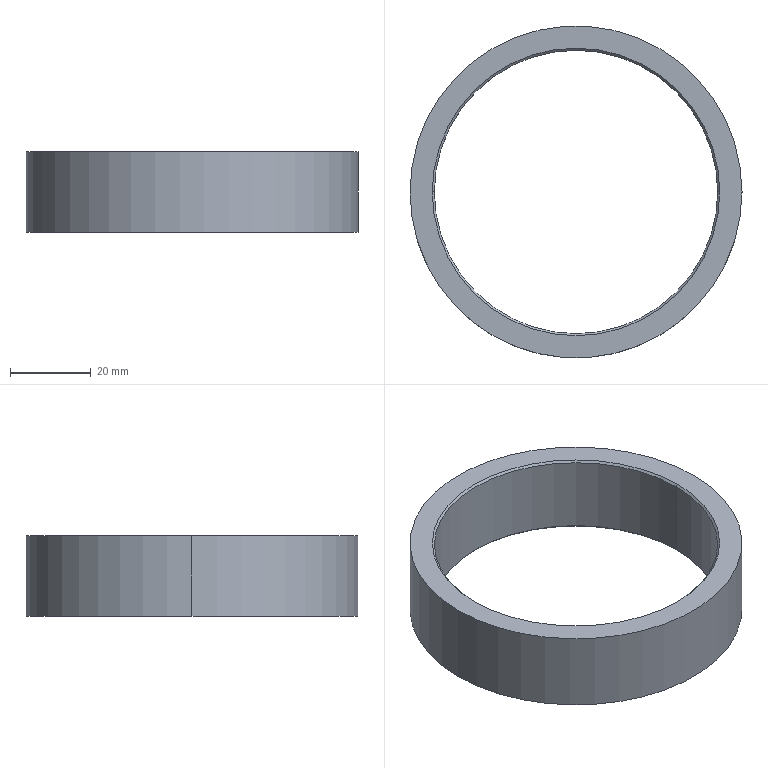Part | SolidWorks | features Chamfer 1, Extrusion 1 | 1 solid | 10 faces | box 82 x 82 x 20 mm | volume 28596 mm3 | cone 4 | cylinder 4 | plane 2 | commonest cylinder face diameters 70 x2 82 x2
STEP:
#1=CARTESIAN_POINT('',(35.,0.,0.5));
#2=VERTEX_POINT('',#1);
#3=CARTESIAN_POINT('',(-35.,0.,0.5));
#4=VERTEX_POINT('',#3);
#5=CARTESIAN_POINT('',(0.,0.,0.5));
#6=DIRECTION('',(0.,0.,-1.));
#7=DIRECTION('',(1.,0.,0.));
#8=AXIS2_PLACEMENT_3D('',#5,#6,#7);
#9=CIRCLE('',#8,35.);
#10=EDGE_CURVE('',#2,#4,#9,.T.);
#11=ORIENTED_EDGE('',*,*,#10,.F.);
#12=CARTESIAN_POINT('',(35.5,0.,0.));
#13=VERTEX_POINT('',#12);
#14=CARTESIAN_POINT('',(35.5,0.,0.));
#15=DIRECTION('',(0.7071,0.,-0.7071));
#16=VECTOR('',#15,1000.);
#17=LINE('',#14,#16);
#18=EDGE_CURVE('',#2,#13,#17,.T.);
#19=ORIENTED_EDGE('',*,*,#18,.T.);
#20=CARTESIAN_POINT('',(-35.5,0.,0.));
#21=VERTEX_POINT('',#20);
#22=CARTESIAN_POINT('',(0.,0.,0.));
#23=DIRECTION('',(0.,0.,1.));
#24=DIRECTION('',(1.,0.,0.));
#25=AXIS2_PLACEMENT_3D('',#22,#23,#24);
#26=CIRCLE('',#25,35.5);
#27=EDGE_CURVE('',#21,#13,#26,.T.);
#28=ORIENTED_EDGE('',*,*,#27,.F.);
#29=CARTESIAN_POINT('',(-35.5,0.,0.));
#30=DIRECTION('',(-0.7071,0.,-0.7071));
#31=VECTOR('',#30,1000.);
#32=LINE('',#29,#31);
#33=EDGE_CURVE('',#4,#21,#32,.T.);
#34=ORIENTED_EDGE('',*,*,#33,.F.);
#35=EDGE_LOOP('',(#11,#19,#28,#34));
#36=FACE_OUTER_BOUND('',#35,.T.);
#37=CARTESIAN_POINT('',(0.,0.,0.));
#38=DIRECTION('',(0.,0.,-1.));
#39=DIRECTION('',(-1.,0.,0.));
#40=AXIS2_PLACEMENT_3D('',#37,#38,#39);
#41=CONICAL_SURFACE('',#40,35.5,0.7854);
#42=ADVANCED_FACE('',(#36),#41,.F.);
#43=CARTESIAN_POINT('',(-35.,0.,19.5));
#44=VERTEX_POINT('',#43);
#45=CARTESIAN_POINT('',(35.,0.,19.5));
#46=VERTEX_POINT('',#45);
#47=CARTESIAN_POINT('',(0.,0.,19.5));
#48=DIRECTION('',(0.,0.,1.));
#49=DIRECTION('',(1.,0.,0.));
#50=AXIS2_PLACEMENT_3D('',#47,#48,#49);
#51=CIRCLE('',#50,35.);
#52=EDGE_CURVE('',#44,#46,#51,.T.);
#53=ORIENTED_EDGE('',*,*,#52,.F.);
#54=CARTESIAN_POINT('',(-35.5,0.,20.));
#55=VERTEX_POINT('',#54);
#56=CARTESIAN_POINT('',(-35.,0.,19.5));
#57=DIRECTION('',(-0.7071,0.,0.7071));
#58=VECTOR('',#57,1000.);
#59=LINE('',#56,#58);
#60=EDGE_CURVE('',#44,#55,#59,.T.);
#61=ORIENTED_EDGE('',*,*,#60,.T.);
#62=CARTESIAN_POINT('',(35.5,0.,20.));
#63=VERTEX_POINT('',#62);
#64=CARTESIAN_POINT('',(0.,0.,20.));
#65=DIRECTION('',(0.,0.,-1.));
#66=DIRECTION('',(1.,0.,0.));
#67=AXIS2_PLACEMENT_3D('',#64,#65,#66);
#68=CIRCLE('',#67,35.5);
#69=EDGE_CURVE('',#63,#55,#68,.T.);
#70=ORIENTED_EDGE('',*,*,#69,.F.);
#71=CARTESIAN_POINT('',(35.,0.,19.5));
#72=DIRECTION('',(0.7071,0.,0.7071));
#73=VECTOR('',#72,1000.);
#74=LINE('',#71,#73);
#75=EDGE_CURVE('',#46,#63,#74,.T.);
#76=ORIENTED_EDGE('',*,*,#75,.F.);
#77=EDGE_LOOP('',(#53,#61,#70,#76));
#78=FACE_OUTER_BOUND('',#77,.T.);
#79=CARTESIAN_POINT('',(0.,0.,19.5));
#80=DIRECTION('',(0.,0.,1.));
#81=DIRECTION('',(1.,0.,0.));
#82=AXIS2_PLACEMENT_3D('',#79,#80,#81);
#83=CONICAL_SURFACE('',#82,35.,0.7854);
#84=ADVANCED_FACE('',(#78),#83,.F.);
#85=ORIENTED_EDGE('',*,*,#52,.T.);
#86=CARTESIAN_POINT('',(35.,0.,20.));
#87=DIRECTION('',(0.,0.,-1.));
#88=VECTOR('',#87,1000.);
#89=LINE('',#86,#88);
#90=EDGE_CURVE('',#46,#2,#89,.T.);
#91=ORIENTED_EDGE('',*,*,#90,.T.);
#92=ORIENTED_EDGE('',*,*,#10,.T.);
#93=CARTESIAN_POINT('',(-35.,0.,20.));
#94=DIRECTION('',(0.,0.,-1.));
#95=VECTOR('',#94,1000.);
#96=LINE('',#93,#95);
#97=EDGE_CURVE('',#44,#4,#96,.T.);
#98=ORIENTED_EDGE('',*,*,#97,.F.);
#99=EDGE_LOOP('',(#85,#91,#92,#98));
#100=FACE_OUTER_BOUND('',#99,.T.);
#101=CARTESIAN_POINT('',(0.,0.,20.));
#102=DIRECTION('',(0.,0.,-1.));
#103=DIRECTION('',(-1.,0.,0.));
#104=AXIS2_PLACEMENT_3D('',#101,#102,#103);
#105=CYLINDRICAL_SURFACE('',#104,35.);
#106=ADVANCED_FACE('',(#100),#105,.F.);
#107=CARTESIAN_POINT('',(41.,0.,20.));
#108=VERTEX_POINT('',#107);
#109=CARTESIAN_POINT('',(-41.,0.,20.));
#110=VERTEX_POINT('',#109);
#111=CARTESIAN_POINT('',(0.,0.,20.));
#112=DIRECTION('',(0.,0.,1.));
#113=DIRECTION('',(1.,0.,0.));
#114=AXIS2_PLACEMENT_3D('',#111,#112,#113);
#115=CIRCLE('',#114,41.);
#116=EDGE_CURVE('',#108,#110,#115,.T.);
#117=ORIENTED_EDGE('',*,*,#116,.F.);
#118=CARTESIAN_POINT('',(41.,0.,0.));
#119=VERTEX_POINT('',#118);
#120=CARTESIAN_POINT('',(41.,0.,20.));
#121=DIRECTION('',(0.,0.,-1.));
#122=VECTOR('',#121,1000.);
#123=LINE('',#120,#122);
#124=EDGE_CURVE('',#108,#119,#123,.T.);
#125=ORIENTED_EDGE('',*,*,#124,.T.);
#126=CARTESIAN_POINT('',(-41.,0.,0.));
#127=VERTEX_POINT('',#126);
#128=CARTESIAN_POINT('',(0.,0.,0.));
#129=DIRECTION('',(0.,0.,1.));
#130=DIRECTION('',(1.,0.,0.));
#131=AXIS2_PLACEMENT_3D('',#128,#129,#130);
#132=CIRCLE('',#131,41.);
#133=EDGE_CURVE('',#119,#127,#132,.T.);
#134=ORIENTED_EDGE('',*,*,#133,.T.);
#135=CARTESIAN_POINT('',(-41.,0.,20.));
#136=DIRECTION('',(0.,0.,-1.));
#137=VECTOR('',#136,1000.);
#138=LINE('',#135,#137);
#139=EDGE_CURVE('',#110,#127,#138,.T.);
#140=ORIENTED_EDGE('',*,*,#139,.F.);
#141=EDGE_LOOP('',(#117,#125,#134,#140));
#142=FACE_OUTER_BOUND('',#141,.T.);
#143=CARTESIAN_POINT('',(0.,0.,20.));
#144=DIRECTION('',(0.,0.,-1.));
#145=DIRECTION('',(-1.,0.,0.));
#146=AXIS2_PLACEMENT_3D('',#143,#144,#145);
#147=CYLINDRICAL_SURFACE('',#146,41.);
#148=ADVANCED_FACE('',(#142),#147,.T.);
#149=ORIENTED_EDGE('',*,*,#69,.T.);
#150=CARTESIAN_POINT('',(0.,0.,20.));
#151=DIRECTION('',(0.,0.,-1.));
#152=DIRECTION('',(1.,0.,0.));
#153=AXIS2_PLACEMENT_3D('',#150,#151,#152);
#154=CIRCLE('',#153,35.5);
#155=EDGE_CURVE('',#55,#63,#154,.T.);
#156=ORIENTED_EDGE('',*,*,#155,.T.);
#157=EDGE_LOOP('',(#149,#156));
#158=FACE_BOUND('',#157,.T.);
#159=CARTESIAN_POINT('',(0.,0.,20.));
#160=DIRECTION('',(0.,0.,1.));
#161=DIRECTION('',(1.,0.,0.));
#162=AXIS2_PLACEMENT_3D('',#159,#160,#161);
#163=CIRCLE('',#162,41.);
#164=EDGE_CURVE('',#110,#108,#163,.T.);
#165=ORIENTED_EDGE('',*,*,#164,.T.);
#166=ORIENTED_EDGE('',*,*,#116,.T.);
#167=EDGE_LOOP('',(#165,#166));
#168=FACE_OUTER_BOUND('',#167,.T.);
#169=CARTESIAN_POINT('',(0.,0.,20.));
#170=DIRECTION('',(0.,0.,1.));
#171=DIRECTION('',(1.,0.,0.));
#172=AXIS2_PLACEMENT_3D('',#169,#170,#171);
#173=PLANE('',#172);
#174=ADVANCED_FACE('',(#158,#168),#173,.T.);
#175=ORIENTED_EDGE('',*,*,#27,.T.);
#176=CARTESIAN_POINT('',(0.,0.,0.));
#177=DIRECTION('',(0.,0.,1.));
#178=DIRECTION('',(1.,0.,0.));
#179=AXIS2_PLACEMENT_3D('',#176,#177,#178);
#180=CIRCLE('',#179,35.5);
#181=EDGE_CURVE('',#13,#21,#180,.T.);
#182=ORIENTED_EDGE('',*,*,#181,.T.);
#183=EDGE_LOOP('',(#175,#182));
#184=FACE_BOUND('',#183,.T.);
#185=CARTESIAN_POINT('',(0.,0.,0.));
#186=DIRECTION('',(0.,0.,1.));
#187=DIRECTION('',(1.,0.,0.));
#188=AXIS2_PLACEMENT_3D('',#185,#186,#187);
#189=CIRCLE('',#188,41.);
#190=EDGE_CURVE('',#127,#119,#189,.T.);
#191=ORIENTED_EDGE('',*,*,#190,.F.);
#192=ORIENTED_EDGE('',*,*,#133,.F.);
#193=EDGE_LOOP('',(#191,#192));
#194=FACE_OUTER_BOUND('',#193,.T.);
#195=CARTESIAN_POINT('',(0.,0.,0.));
#196=DIRECTION('',(0.,0.,1.));
#197=DIRECTION('',(1.,0.,0.));
#198=AXIS2_PLACEMENT_3D('',#195,#196,#197);
#199=PLANE('',#198);
#200=ADVANCED_FACE('',(#184,#194),#199,.F.);
#201=ORIENTED_EDGE('',*,*,#124,.F.);
#202=ORIENTED_EDGE('',*,*,#164,.F.);
#203=ORIENTED_EDGE('',*,*,#139,.T.);
#204=ORIENTED_EDGE('',*,*,#190,.T.);
#205=EDGE_LOOP('',(#201,#202,#203,#204));
#206=FACE_OUTER_BOUND('',#205,.T.);
#207=CARTESIAN_POINT('',(0.,0.,20.));
#208=DIRECTION('',(0.,0.,-1.));
#209=DIRECTION('',(-1.,0.,0.));
#210=AXIS2_PLACEMENT_3D('',#207,#208,#209);
#211=CYLINDRICAL_SURFACE('',#210,41.);
#212=ADVANCED_FACE('',(#206),#211,.T.);
#213=ORIENTED_EDGE('',*,*,#90,.F.);
#214=CARTESIAN_POINT('',(0.,0.,19.5));
#215=DIRECTION('',(0.,0.,1.));
#216=DIRECTION('',(1.,0.,0.));
#217=AXIS2_PLACEMENT_3D('',#214,#215,#216);
#218=CIRCLE('',#217,35.);
#219=EDGE_CURVE('',#46,#44,#218,.T.);
#220=ORIENTED_EDGE('',*,*,#219,.T.);
#221=ORIENTED_EDGE('',*,*,#97,.T.);
#222=CARTESIAN_POINT('',(0.,0.,0.5));
#223=DIRECTION('',(0.,0.,-1.));
#224=DIRECTION('',(1.,0.,0.));
#225=AXIS2_PLACEMENT_3D('',#222,#223,#224);
#226=CIRCLE('',#225,35.);
#227=EDGE_CURVE('',#4,#2,#226,.T.);
#228=ORIENTED_EDGE('',*,*,#227,.T.);
#229=EDGE_LOOP('',(#213,#220,#221,#228));
#230=FACE_OUTER_BOUND('',#229,.T.);
#231=CARTESIAN_POINT('',(0.,0.,20.));
#232=DIRECTION('',(0.,0.,-1.));
#233=DIRECTION('',(-1.,0.,0.));
#234=AXIS2_PLACEMENT_3D('',#231,#232,#233);
#235=CYLINDRICAL_SURFACE('',#234,35.);
#236=ADVANCED_FACE('',(#230),#235,.F.);
#237=ORIENTED_EDGE('',*,*,#60,.F.);
#238=ORIENTED_EDGE('',*,*,#219,.F.);
#239=ORIENTED_EDGE('',*,*,#75,.T.);
#240=ORIENTED_EDGE('',*,*,#155,.F.);
#241=EDGE_LOOP('',(#237,#238,#239,#240));
#242=FACE_OUTER_BOUND('',#241,.T.);
#243=CARTESIAN_POINT('',(0.,0.,19.5));
#244=DIRECTION('',(0.,0.,1.));
#245=DIRECTION('',(1.,0.,0.));
#246=AXIS2_PLACEMENT_3D('',#243,#244,#245);
#247=CONICAL_SURFACE('',#246,35.,0.7854);
#248=ADVANCED_FACE('',(#242),#247,.F.);
#249=ORIENTED_EDGE('',*,*,#18,.F.);
#250=ORIENTED_EDGE('',*,*,#227,.F.);
#251=ORIENTED_EDGE('',*,*,#33,.T.);
#252=ORIENTED_EDGE('',*,*,#181,.F.);
#253=EDGE_LOOP('',(#249,#250,#251,#252));
#254=FACE_OUTER_BOUND('',#253,.T.);
#255=CARTESIAN_POINT('',(0.,0.,0.));
#256=DIRECTION('',(0.,0.,-1.));
#257=DIRECTION('',(-1.,0.,0.));
#258=AXIS2_PLACEMENT_3D('',#255,#256,#257);
#259=CONICAL_SURFACE('',#258,35.5,0.7854);
#260=ADVANCED_FACE('',(#254),#259,.F.);
#261=CLOSED_SHELL('',(#42,#84,#106,#148,#174,#200,#212,#236,#248,#260));
#262=MANIFOLD_SOLID_BREP('',#261);
#263=CARTESIAN_POINT('',(0.,0.,0.));
#264=DIRECTION('',(0.,0.,1.));
#265=DIRECTION('',(1.,0.,0.));
#266=AXIS2_PLACEMENT_3D('',#263,#264,#265);
#267=(LENGTH_UNIT()NAMED_UNIT(*)SI_UNIT(.MILLI.,.METRE.));
#268=UNCERTAINTY_MEASURE_WITH_UNIT(LENGTH_MEASURE(0.00001),#267,'','');
#269=(NAMED_UNIT(*)PLANE_ANGLE_UNIT()SI_UNIT($,.RADIAN.));
#270=(NAMED_UNIT(*)SI_UNIT($,.STERADIAN.)SOLID_ANGLE_UNIT());
#271=(GEOMETRIC_REPRESENTATION_CONTEXT(3)GLOBAL_UNCERTAINTY_ASSIGNED_CONTEXT((#268))GLOBAL_UNIT_ASSIGNED_CONTEXT((#267,#269,#270))REPRESENTATION_CONTEXT('',''));
#272=ADVANCED_BREP_SHAPE_REPRESENTATION('',(#262,#266),#271);